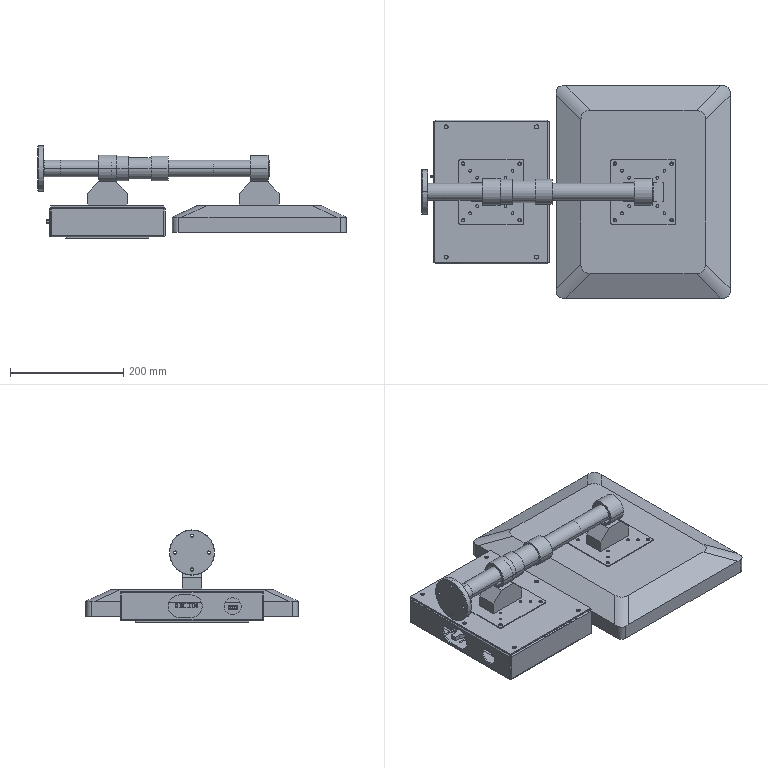Part | SolidWorks | 8 solids | 435 faces | box 544.678 x 375 x 163 mm | volume 5912410 mm3 | plane 203 | cylinder 198 | spline 16 | cone 14 | sphere 4 | commonest cylinder face diameters 5 x68 6 x28 4 x20 7 x12 1 x8 5.5 x8